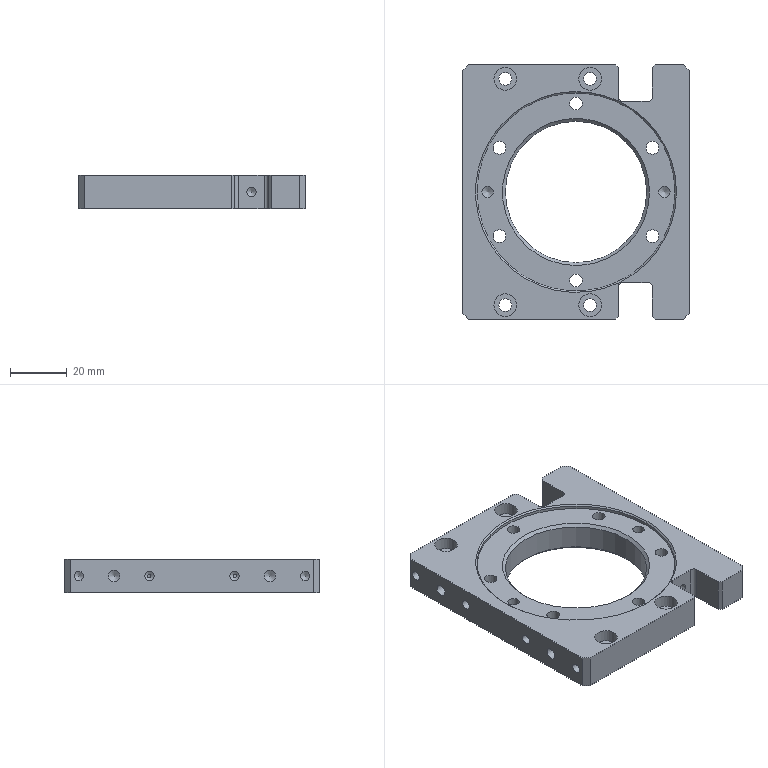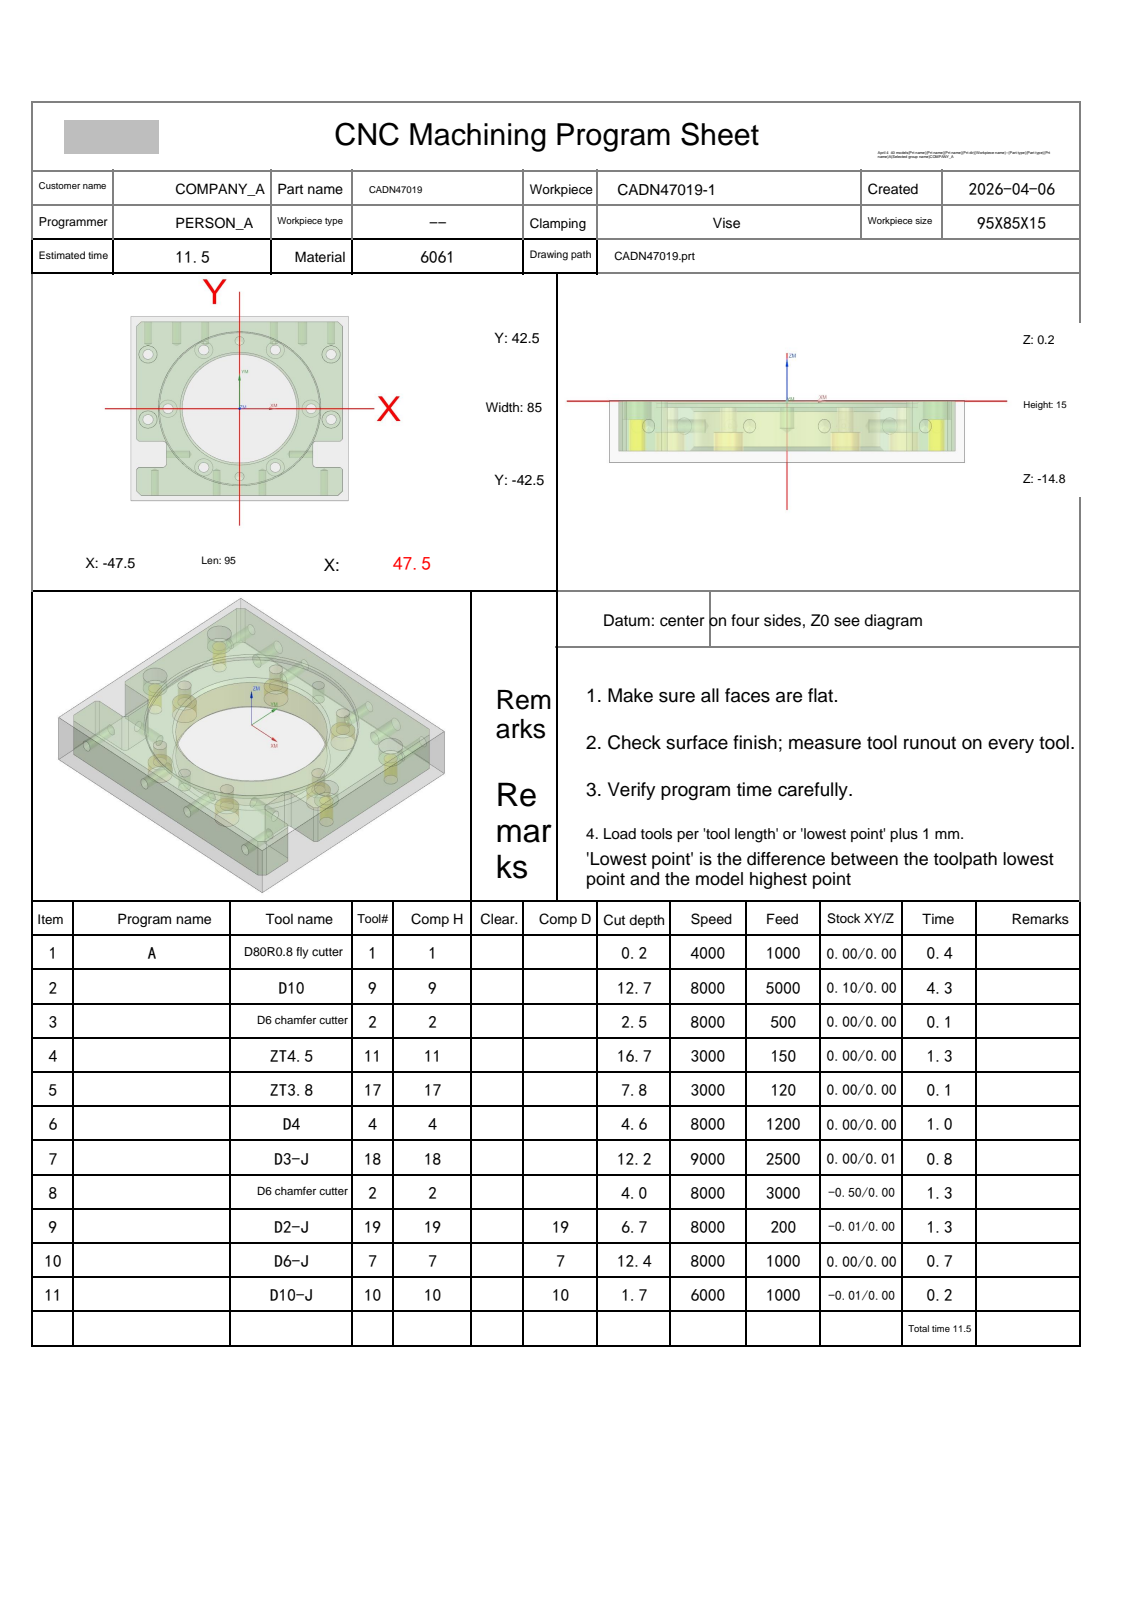NC program | NX | posted by the shop | part box 80 x 90 x 12 mm
Lines 2082 to 3119 of 6628:
N7 T18 M06
(D3-J  D=3. R=0. H=18 ce=0.00 di=0.01)
G00 G90 G54 X37.397 Y-17.082 M03 S9000
G43 H18 Z20.
M08
Z.151
G01 Y-17.076 Z.083 F2000.
X37.394 Y-17.059 Z.021
X37.39 Y-17.032 Z-.034
X37.384 Y-16.996 Z-.083
X37.375 Y-16.954 Z-.125
X37.364 Y-16.907 Z-.163
X37.351 Y-16.856 Z-.195
X37.334 Y-16.803 Z-.222
X37.315 Y-16.749 Z-.244
X37.293 Y-16.696 Z-.262
X37.267 Y-16.646 Z-.276
X37.237 Y-16.6 Z-.287
X37.204 Y-16.559 Z-.294
X37.167 Y-16.525 Z-.297
X37.125 Y-16.5 Z-.299
X33.5 F2500.
Y-20.125
X33.516 Y-20.154 Z-.3
X33.561 Y-20.159 Z-.302
X33.633 Y-20.143 Z-.306
X33.728 Y-20.106 Z-.312
X33.843 Y-20.052 Z-.319
X33.975 Y-19.981 Z-.327
X34.273 Y-19.8 Z-.346
X34.466 Y-19.672 Z-.358
X34.779 Y-19.448 Z-.38
X35.235 Y-19.077 Z-.413
X35.669 Y-18.672 Z-.448
X36.075 Y-18.238 Z-.483
X36.447 Y-17.781 Z-.517
X36.671 Y-17.468 Z-.538
X36.8 Y-17.275 Z-.55
X36.981 Y-16.976 Z-.569
X37.052 Y-16.844 Z-.577
X37.106 Y-16.729 Z-.584
X37.142 Y-16.633 Z-.59
X37.159 Y-16.561 Z-.594
X37.154 Y-16.516 Z-.597
X37.125 Y-16.5 Z-.598
X33.5
Y-20.125
X33.516 Y-20.154
X33.561 Y-20.159 Z-.601
X33.633 Y-20.143 Z-.605
X33.728 Y-20.106 Z-.611
X33.843 Y-20.052 Z-.618
X33.975 Y-19.981 Z-.626
X34.273 Y-19.8 Z-.645
X34.466 Y-19.672 Z-.657
X34.779 Y-19.448 Z-.678
X35.235 Y-19.077 Z-.712
X35.669 Y-18.672 Z-.747
X36.075 Y-18.238 Z-.782
X36.447 Y-17.781 Z-.815
X36.671 Y-17.468 Z-.837
X36.8 Y-17.275 Z-.849
X36.981 Y-16.976 Z-.868
X37.052 Y-16.844 Z-.876
X37.106 Y-16.729 Z-.883
X37.142 Y-16.633 Z-.889
X37.159 Y-16.561 Z-.893
X37.154 Y-16.516 Z-.895
X37.125 Y-16.5 Z-.896
X33.5
Y-20.125
X33.516 Y-20.154 Z-.897
X33.561 Y-20.159 Z-.9
X33.633 Y-20.143 Z-.904
X33.728 Y-20.106 Z-.91
X33.843 Y-20.052 Z-.916
X33.975 Y-19.981 Z-.925
X34.273 Y-19.8 Z-.943
X34.466 Y-19.672 Z-.956
X34.779 Y-19.448 Z-.977
X35.235 Y-19.077 Z-1.011
X35.669 Y-18.672 Z-1.046
X36.075 Y-18.238 Z-1.08
X36.447 Y-17.781 Z-1.114
X36.671 Y-17.468 Z-1.135
X36.8 Y-17.275 Z-1.148
X36.981 Y-16.976 Z-1.167
X37.052 Y-16.844 Z-1.175
X37.106 Y-16.729 Z-1.182
X37.142 Y-16.633 Z-1.187
X37.159 Y-16.561 Z-1.191
X37.154 Y-16.516 Z-1.194
X37.125 Y-16.5 Z-1.195
X33.5
Y-20.125
X33.516 Y-20.154 Z-1.196
X33.561 Y-20.159 Z-1.199
X33.633 Y-20.143 Z-1.203
X33.728 Y-20.106 Z-1.208
X33.843 Y-20.052 Z-1.215
X33.975 Y-19.981 Z-1.223
X34.273 Y-19.8 Z-1.242
X34.466 Y-19.672 Z-1.255
X34.779 Y-19.448 Z-1.276
X35.235 Y-19.077 Z-1.31
X35.669 Y-18.672 Z-1.344
X36.075 Y-18.238 Z-1.379
X36.447 Y-17.781 Z-1.413
X36.671 Y-17.468 Z-1.434
X36.8 Y-17.275 Z-1.447
X36.981 Y-16.976 Z-1.465
X37.052 Y-16.844 Z-1.474
X37.106 Y-16.729 Z-1.48
X37.142 Y-16.633 Z-1.486
X37.159 Y-16.561 Z-1.49
X37.154 Y-16.516 Z-1.493
X37.125 Y-16.5 Z-1.494
X33.5
Y-20.125
X33.516 Y-20.154 Z-1.495
X33.561 Y-20.159 Z-1.497
X33.633 Y-20.143 Z-1.501
X33.728 Y-20.106 Z-1.507
X33.843 Y-20.052 Z-1.514
X33.975 Y-19.981 Z-1.522
X34.273 Y-19.8 Z-1.541
X34.466 Y-19.672 Z-1.553
X34.779 Y-19.448 Z-1.575
X35.235 Y-19.077 Z-1.608
X35.669 Y-18.672 Z-1.643
X36.075 Y-18.238 Z-1.678
X36.447 Y-17.781 Z-1.712
X36.671 Y-17.468 Z-1.733
X36.8 Y-17.275 Z-1.745
X36.981 Y-16.976 Z-1.764
X37.052 Y-16.844 Z-1.772
X37.106 Y-16.729 Z-1.779
X37.142 Y-16.633 Z-1.785
X37.159 Y-16.561 Z-1.789
X37.154 Y-16.516 Z-1.792
X37.125 Y-16.5 Z-1.793
X33.5
Y-20.125
X33.516 Y-20.154
X33.561 Y-20.159 Z-1.796
X33.633 Y-20.143 Z-1.8
X33.728 Y-20.106 Z-1.806
X33.843 Y-20.052 Z-1.813
X33.975 Y-19.981 Z-1.821
X34.273 Y-19.8 Z-1.84
X34.466 Y-19.672 Z-1.852
X34.779 Y-19.448 Z-1.873
X35.235 Y-19.077 Z-1.907
X35.669 Y-18.672 Z-1.942
X36.075 Y-18.238 Z-1.977
X36.447 Y-17.781 Z-2.01
X36.671 Y-17.468 Z-2.032
X36.8 Y-17.275 Z-2.044
X36.981 Y-16.976 Z-2.063
X37.052 Y-16.844 Z-2.071
X37.106 Y-16.729 Z-2.078
X37.142 Y-16.633 Z-2.084
X37.159 Y-16.561 Z-2.088
X37.154 Y-16.516 Z-2.09
X37.125 Y-16.5 Z-2.091
X33.5
Y-20.125
X33.516 Y-20.154 Z-2.092
X33.561 Y-20.159 Z-2.095
X33.633 Y-20.143 Z-2.099
X33.728 Y-20.106 Z-2.105
X33.843 Y-20.052 Z-2.111
X33.975 Y-19.981 Z-2.12
X34.273 Y-19.8 Z-2.138
X34.466 Y-19.672 Z-2.151
X34.779 Y-19.448 Z-2.172
X35.235 Y-19.077 Z-2.206
X35.669 Y-18.672 Z-2.241
X36.075 Y-18.238 Z-2.275
X36.447 Y-17.781 Z-2.309
X36.671 Y-17.468 Z-2.33
X36.8 Y-17.275 Z-2.343
X36.981 Y-16.976 Z-2.362
X37.052 Y-16.844 Z-2.37
X37.106 Y-16.729 Z-2.377
X37.142 Y-16.633 Z-2.382
X37.159 Y-16.561 Z-2.386
X37.154 Y-16.516 Z-2.389
X37.125 Y-16.5 Z-2.39
X33.5
Y-20.125
X33.516 Y-20.154 Z-2.391
X33.561 Y-20.159 Z-2.394
X33.633 Y-20.143 Z-2.398
X33.728 Y-20.106 Z-2.403
X33.843 Y-20.052 Z-2.41
X33.975 Y-19.981 Z-2.418
X34.273 Y-19.8 Z-2.437
X34.466 Y-19.672 Z-2.45
X34.779 Y-19.448 Z-2.471
X35.235 Y-19.077 Z-2.505
X35.669 Y-18.672 Z-2.539
X36.075 Y-18.238 Z-2.574
X36.447 Y-17.781 Z-2.608
X36.671 Y-17.468 Z-2.629
X36.8 Y-17.275 Z-2.642
X36.981 Y-16.976 Z-2.66
X37.052 Y-16.844 Z-2.669
X37.106 Y-16.729 Z-2.675
X37.142 Y-16.633 Z-2.681
X37.159 Y-16.561 Z-2.685
X37.154 Y-16.516 Z-2.688
X37.125 Y-16.5 Z-2.689
X33.5
Y-20.125
X33.516 Y-20.154 Z-2.69
X33.561 Y-20.159 Z-2.692
X33.633 Y-20.143 Z-2.696
X33.728 Y-20.106 Z-2.702
X33.843 Y-20.052 Z-2.709
X33.975 Y-19.981 Z-2.717
X34.273 Y-19.8 Z-2.736
X34.466 Y-19.672 Z-2.748
X34.779 Y-19.448 Z-2.77
X35.235 Y-19.077 Z-2.803
X35.669 Y-18.672 Z-2.838
X36.075 Y-18.238 Z-2.873
X36.447 Y-17.781 Z-2.907
X36.671 Y-17.468 Z-2.928
X36.8 Y-17.275 Z-2.94
X36.981 Y-16.976 Z-2.959
X37.052 Y-16.844 Z-2.967
X37.106 Y-16.729 Z-2.974
X37.142 Y-16.633 Z-2.98
X37.159 Y-16.561 Z-2.984
X37.154 Y-16.516 Z-2.987
X37.125 Y-16.5 Z-2.988
X33.5
Y-20.125
X33.516 Y-20.154
X33.561 Y-20.159 Z-2.991
X33.633 Y-20.143 Z-2.995
X33.728 Y-20.106 Z-3.001
X33.843 Y-20.052 Z-3.008
X33.975 Y-19.981 Z-3.016
X34.273 Y-19.8 Z-3.035
X34.466 Y-19.672 Z-3.047
X34.779 Y-19.448 Z-3.068
X35.235 Y-19.077 Z-3.102
X35.669 Y-18.672 Z-3.137
X36.075 Y-18.238 Z-3.172
X36.447 Y-17.781 Z-3.205
X36.671 Y-17.468 Z-3.227
X36.8 Y-17.275 Z-3.239
X36.981 Y-16.976 Z-3.258
X37.052 Y-16.844 Z-3.266
X37.106 Y-16.729 Z-3.273
X37.142 Y-16.633 Z-3.279
X37.159 Y-16.561 Z-3.283
X37.154 Y-16.516 Z-3.285
X37.125 Y-16.5 Z-3.286
X33.5
Y-20.125
X33.516 Y-20.154 Z-3.287
X33.561 Y-20.159 Z-3.29
X33.633 Y-20.143 Z-3.294
X33.728 Y-20.106 Z-3.3
X33.843 Y-20.052 Z-3.306
X33.975 Y-19.981 Z-3.315
X34.273 Y-19.8 Z-3.333
X34.466 Y-19.672 Z-3.346
X34.779 Y-19.448 Z-3.367
X35.235 Y-19.077 Z-3.401
X35.669 Y-18.672 Z-3.436
X36.075 Y-18.238 Z-3.47
X36.447 Y-17.781 Z-3.504
X36.671 Y-17.468 Z-3.525
X36.8 Y-17.275 Z-3.538
X36.981 Y-16.976 Z-3.557
X37.052 Y-16.844 Z-3.565
X37.106 Y-16.729 Z-3.572
X37.142 Y-16.633 Z-3.577
X37.159 Y-16.561 Z-3.581
X37.154 Y-16.516 Z-3.584
X37.125 Y-16.5 Z-3.585
X33.5
Y-20.125
X33.516 Y-20.154 Z-3.586
X33.561 Y-20.159 Z-3.589
X33.633 Y-20.143 Z-3.593
X33.728 Y-20.106 Z-3.598
X33.843 Y-20.052 Z-3.605
X33.975 Y-19.981 Z-3.613
X34.273 Y-19.8 Z-3.632
X34.466 Y-19.672 Z-3.645
X34.779 Y-19.448 Z-3.666
X35.235 Y-19.077 Z-3.7
X35.669 Y-18.672 Z-3.734
X36.075 Y-18.238 Z-3.769
X36.447 Y-17.781 Z-3.803
X36.671 Y-17.468 Z-3.824
X36.8 Y-17.275 Z-3.837
X36.981 Y-16.976 Z-3.855
X37.052 Y-16.844 Z-3.864
X37.106 Y-16.729 Z-3.87
X37.142 Y-16.633 Z-3.876
X37.159 Y-16.561 Z-3.88
X37.154 Y-16.516 Z-3.883
X37.125 Y-16.5 Z-3.884
X33.5
Y-20.125
X33.516 Y-20.154 Z-3.885
X33.561 Y-20.159 Z-3.887
X33.633 Y-20.143 Z-3.891
X33.728 Y-20.106 Z-3.897
X33.843 Y-20.052 Z-3.904
X33.975 Y-19.981 Z-3.912
X34.273 Y-19.8 Z-3.931
X34.466 Y-19.672 Z-3.943
X34.779 Y-19.448 Z-3.965
X35.235 Y-19.077 Z-3.998
X35.669 Y-18.672 Z-4.033
X36.075 Y-18.238 Z-4.068
X36.447 Y-17.781 Z-4.102
X36.671 Y-17.468 Z-4.123
X36.8 Y-17.275 Z-4.135
X36.981 Y-16.976 Z-4.154
X37.052 Y-16.844 Z-4.162
X37.106 Y-16.729 Z-4.169
X37.142 Y-16.633 Z-4.175
X37.159 Y-16.561 Z-4.179
X37.154 Y-16.516 Z-4.182
X37.125 Y-16.5 Z-4.183
X33.5
Y-20.125
X33.516 Y-20.154
X33.561 Y-20.159 Z-4.186
X33.633 Y-20.143 Z-4.19
X33.728 Y-20.106 Z-4.196
X33.843 Y-20.052 Z-4.203
X33.975 Y-19.981 Z-4.211
X34.273 Y-19.8 Z-4.23
X34.466 Y-19.672 Z-4.242
X34.779 Y-19.448 Z-4.263
X35.235 Y-19.077 Z-4.297
X35.669 Y-18.672 Z-4.332
X36.075 Y-18.238 Z-4.367
X36.447 Y-17.781 Z-4.4
X36.671 Y-17.468 Z-4.422
X36.8 Y-17.275 Z-4.434
X36.981 Y-16.976 Z-4.453
X37.052 Y-16.844 Z-4.461
X37.106 Y-16.729 Z-4.468
X37.142 Y-16.633 Z-4.474
X37.159 Y-16.561 Z-4.478
X37.154 Y-16.516 Z-4.48
X37.125 Y-16.5 Z-4.481
X33.5
Y-20.125
X33.516 Y-20.154 Z-4.482
X33.561 Y-20.159 Z-4.485
X33.633 Y-20.143 Z-4.489
X33.728 Y-20.106 Z-4.495
X33.843 Y-20.052 Z-4.501
X33.975 Y-19.981 Z-4.51
X34.273 Y-19.8 Z-4.528
X34.466 Y-19.672 Z-4.541
X34.779 Y-19.448 Z-4.562
X35.235 Y-19.077 Z-4.596
X35.669 Y-18.672 Z-4.631
X36.075 Y-18.238 Z-4.665
X36.447 Y-17.781 Z-4.699
X36.671 Y-17.468 Z-4.72
X36.8 Y-17.275 Z-4.733
X36.981 Y-16.976 Z-4.752
X37.052 Y-16.844 Z-4.76
X37.106 Y-16.729 Z-4.767
X37.142 Y-16.633 Z-4.772
X37.159 Y-16.561 Z-4.776
X37.154 Y-16.516 Z-4.779
X37.125 Y-16.5 Z-4.78
X33.5
Y-20.125
X33.516 Y-20.154 Z-4.781
X33.561 Y-20.159 Z-4.784
X33.633 Y-20.143 Z-4.788
X33.728 Y-20.106 Z-4.793
X33.843 Y-20.052 Z-4.8
X33.975 Y-19.981 Z-4.808
X34.273 Y-19.8 Z-4.827
X34.466 Y-19.672 Z-4.84
X34.779 Y-19.448 Z-4.861
X35.235 Y-19.077 Z-4.895
X35.669 Y-18.672 Z-4.929
X36.075 Y-18.238 Z-4.964
X36.447 Y-17.781 Z-4.998
X36.671 Y-17.468 Z-5.019
X36.8 Y-17.275 Z-5.032
X36.981 Y-16.976 Z-5.05
X37.052 Y-16.844 Z-5.059
X37.106 Y-16.729 Z-5.065
X37.142 Y-16.633 Z-5.071
X37.159 Y-16.561 Z-5.075
X37.154 Y-16.516 Z-5.078
X37.125 Y-16.5 Z-5.079
X33.5
Y-20.125
X33.516 Y-20.154 Z-5.08
X33.561 Y-20.159 Z-5.082
X33.633 Y-20.143 Z-5.086
X33.728 Y-20.106 Z-5.092
X33.843 Y-20.052 Z-5.099
X33.975 Y-19.981 Z-5.107
X34.273 Y-19.8 Z-5.126
X34.466 Y-19.672 Z-5.138
X34.779 Y-19.448 Z-5.16
X35.235 Y-19.077 Z-5.193
X35.669 Y-18.672 Z-5.228
X36.075 Y-18.238 Z-5.263
X36.447 Y-17.781 Z-5.297
X36.671 Y-17.468 Z-5.318
X36.8 Y-17.275 Z-5.33
X36.981 Y-16.976 Z-5.349
X37.052 Y-16.844 Z-5.357
X37.106 Y-16.729 Z-5.364
X37.142 Y-16.633 Z-5.37
X37.159 Y-16.561 Z-5.374
X37.154 Y-16.516 Z-5.377
X37.125 Y-16.5 Z-5.378
X33.5
Y-20.125
X33.516 Y-20.154
X33.561 Y-20.159 Z-5.381
X33.633 Y-20.143 Z-5.385
X33.728 Y-20.106 Z-5.391
X33.843 Y-20.052 Z-5.398
X33.975 Y-19.981 Z-5.406
X34.273 Y-19.8 Z-5.425
X34.466 Y-19.672 Z-5.437
X34.779 Y-19.448 Z-5.458
X35.235 Y-19.077 Z-5.492
X35.669 Y-18.672 Z-5.527
X36.075 Y-18.238 Z-5.562
X36.447 Y-17.781 Z-5.595
X36.671 Y-17.468 Z-5.617
X36.8 Y-17.275 Z-5.629
X36.981 Y-16.976 Z-5.648
X37.052 Y-16.844 Z-5.656
X37.106 Y-16.729 Z-5.663
X37.142 Y-16.633 Z-5.669
X37.159 Y-16.561 Z-5.673
X37.154 Y-16.516 Z-5.675
X37.125 Y-16.5 Z-5.676
X33.5
Y-20.125
X33.516 Y-20.154 Z-5.677
X33.561 Y-20.159 Z-5.68
X33.633 Y-20.143 Z-5.684
X33.728 Y-20.106 Z-5.69
X33.843 Y-20.052 Z-5.696
X33.975 Y-19.981 Z-5.705
X34.273 Y-19.8 Z-5.723
X34.466 Y-19.672 Z-5.736
X34.779 Y-19.448 Z-5.757
X35.235 Y-19.077 Z-5.791
X35.669 Y-18.672 Z-5.826
X36.075 Y-18.238 Z-5.86
X36.447 Y-17.781 Z-5.894
X36.671 Y-17.468 Z-5.915
X36.8 Y-17.275 Z-5.928
X36.981 Y-16.976 Z-5.947
X37.052 Y-16.844 Z-5.955
X37.106 Y-16.729 Z-5.962
X37.142 Y-16.633 Z-5.967
X37.159 Y-16.561 Z-5.971
X37.154 Y-16.516 Z-5.974
X37.125 Y-16.5 Z-5.975
X33.5
Y-20.125
X33.516 Y-20.154 Z-5.976
X33.561 Y-20.159 Z-5.979
X33.633 Y-20.143 Z-5.983
X33.728 Y-20.106 Z-5.988
X33.843 Y-20.052 Z-5.995
X33.975 Y-19.981 Z-6.003
X34.273 Y-19.8 Z-6.022
X34.466 Y-19.672 Z-6.035
X34.779 Y-19.448 Z-6.056
X35.235 Y-19.077 Z-6.09
X35.669 Y-18.672 Z-6.124
X36.075 Y-18.238 Z-6.159
X36.447 Y-17.781 Z-6.193
X36.671 Y-17.468 Z-6.214
X36.8 Y-17.275 Z-6.227
X36.981 Y-16.976 Z-6.245
X37.052 Y-16.844 Z-6.254
X37.106 Y-16.729 Z-6.26
X37.142 Y-16.633 Z-6.266
X37.159 Y-16.561 Z-6.27
X37.154 Y-16.516 Z-6.273
X37.125 Y-16.5 Z-6.274
X33.5
Y-20.125
X33.516 Y-20.154 Z-6.275
X33.561 Y-20.159 Z-6.277
X33.633 Y-20.143 Z-6.281
X33.728 Y-20.106 Z-6.287
X33.843 Y-20.052 Z-6.294
X33.975 Y-19.981 Z-6.302
X34.273 Y-19.8 Z-6.321
X34.466 Y-19.672 Z-6.333
X34.779 Y-19.448 Z-6.355
X35.235 Y-19.077 Z-6.388
X35.669 Y-18.672 Z-6.423
X36.075 Y-18.238 Z-6.458
X36.447 Y-17.781 Z-6.492
X36.671 Y-17.468 Z-6.513
X36.8 Y-17.275 Z-6.525
X36.981 Y-16.976 Z-6.544
X37.052 Y-16.844 Z-6.552
X37.106 Y-16.729 Z-6.559
X37.142 Y-16.633 Z-6.565
X37.159 Y-16.561 Z-6.569
X37.154 Y-16.516 Z-6.572
X37.125 Y-16.5 Z-6.573
X33.5
Y-20.125
X33.516 Y-20.154
X33.561 Y-20.159 Z-6.576
X33.633 Y-20.143 Z-6.58
X33.728 Y-20.106 Z-6.586
X33.843 Y-20.052 Z-6.593
X33.975 Y-19.981 Z-6.601
X34.273 Y-19.8 Z-6.62
X34.466 Y-19.672 Z-6.632
X34.779 Y-19.448 Z-6.653
X35.235 Y-19.077 Z-6.687
X35.669 Y-18.672 Z-6.722
X36.075 Y-18.238 Z-6.757
X36.447 Y-17.781 Z-6.79
X36.671 Y-17.468 Z-6.812
X36.8 Y-17.275 Z-6.824
X36.981 Y-16.976 Z-6.843
X37.052 Y-16.844 Z-6.851
X37.106 Y-16.729 Z-6.858
X37.142 Y-16.633 Z-6.864
X37.159 Y-16.561 Z-6.868
X37.154 Y-16.516 Z-6.87
X37.125 Y-16.5 Z-6.871
X33.5
Y-20.125
X33.516 Y-20.154 Z-6.872
X33.561 Y-20.159 Z-6.875
X33.633 Y-20.143 Z-6.879
X33.728 Y-20.106 Z-6.885
X33.843 Y-20.052 Z-6.891
X33.975 Y-19.981 Z-6.9
X34.273 Y-19.8 Z-6.918
X34.466 Y-19.672 Z-6.931
X34.779 Y-19.448 Z-6.952
X35.235 Y-19.077 Z-6.986
X35.669 Y-18.672 Z-7.021
X36.075 Y-18.238 Z-7.055
X36.447 Y-17.781 Z-7.089
X36.671 Y-17.468 Z-7.11
X36.8 Y-17.275 Z-7.123
X36.981 Y-16.976 Z-7.142
X37.052 Y-16.844 Z-7.15
X37.106 Y-16.729 Z-7.157
X37.142 Y-16.633 Z-7.162
X37.159 Y-16.561 Z-7.166
X37.154 Y-16.516 Z-7.169
X37.125 Y-16.5 Z-7.17
X33.5
Y-20.125
X33.516 Y-20.154 Z-7.171
X33.561 Y-20.159 Z-7.174
X33.633 Y-20.143 Z-7.178
X33.728 Y-20.106 Z-7.183
X33.843 Y-20.052 Z-7.19
X33.975 Y-19.981 Z-7.198
X34.273 Y-19.8 Z-7.217
X34.466 Y-19.672 Z-7.23
X34.779 Y-19.448 Z-7.251
X35.235 Y-19.077 Z-7.285
X35.669 Y-18.672 Z-7.319
X36.075 Y-18.238 Z-7.354
X36.447 Y-17.781 Z-7.388
X36.671 Y-17.468 Z-7.409
X36.8 Y-17.275 Z-7.422
X36.981 Y-16.976 Z-7.44
X37.052 Y-16.844 Z-7.449
X37.106 Y-16.729 Z-7.455
X37.142 Y-16.633 Z-7.461
X37.159 Y-16.561 Z-7.465
X37.154 Y-16.516 Z-7.468
X37.125 Y-16.5 Z-7.469
X33.5
Y-20.125
X33.516 Y-20.154 Z-7.47
X33.561 Y-20.159 Z-7.472
X33.633 Y-20.143 Z-7.476
X33.728 Y-20.106 Z-7.482
X33.843 Y-20.052 Z-7.489
X33.975 Y-19.981 Z-7.497
X34.273 Y-19.8 Z-7.516
X34.466 Y-19.672 Z-7.528
X34.779 Y-19.448 Z-7.55
X35.235 Y-19.077 Z-7.583
X35.669 Y-18.672 Z-7.618
X36.075 Y-18.238 Z-7.653
X36.447 Y-17.781 Z-7.687
X36.671 Y-17.468 Z-7.708
X36.8 Y-17.275 Z-7.72
X36.981 Y-16.976 Z-7.739
X37.052 Y-16.844 Z-7.747
X37.106 Y-16.729 Z-7.754
X37.142 Y-16.633 Z-7.76
X37.159 Y-16.561 Z-7.764
X37.154 Y-16.516 Z-7.767
X37.125 Y-16.5 Z-7.768
X33.5
Y-20.125
X33.516 Y-20.154
X33.561 Y-20.159 Z-7.771
X33.633 Y-20.143 Z-7.775
X33.728 Y-20.106 Z-7.781
X33.843 Y-20.052 Z-7.788
X33.975 Y-19.981 Z-7.796
X34.273 Y-19.8 Z-7.815
X34.466 Y-19.672 Z-7.827
X34.779 Y-19.448 Z-7.848
X35.235 Y-19.077 Z-7.882
X35.669 Y-18.672 Z-7.917
X36.075 Y-18.238 Z-7.952
X36.447 Y-17.781 Z-7.985
X36.671 Y-17.468 Z-8.007
X36.8 Y-17.275 Z-8.019
X36.981 Y-16.976 Z-8.038
X37.052 Y-16.844 Z-8.046
X37.106 Y-16.729 Z-8.053
X37.142 Y-16.633 Z-8.059
X37.159 Y-16.561 Z-8.063
X37.154 Y-16.516 Z-8.065
X37.125 Y-16.5 Z-8.066
X33.5
Y-20.125
X33.516 Y-20.154 Z-8.067
X33.561 Y-20.159 Z-8.07
X33.633 Y-20.143 Z-8.074
X33.728 Y-20.106 Z-8.08
X33.843 Y-20.052 Z-8.086
X33.975 Y-19.981 Z-8.095
X34.273 Y-19.8 Z-8.113
X34.466 Y-19.672 Z-8.126
X34.779 Y-19.448 Z-8.147
X35.235 Y-19.077 Z-8.181
X35.669 Y-18.672 Z-8.216
X36.075 Y-18.238 Z-8.25
X36.447 Y-17.781 Z-8.284
X36.671 Y-17.468 Z-8.305
X36.8 Y-17.275 Z-8.318
X36.981 Y-16.976 Z-8.337
X37.052 Y-16.844 Z-8.345
X37.106 Y-16.729 Z-8.352
X37.142 Y-16.633 Z-8.357
X37.159 Y-16.561 Z-8.361
X37.154 Y-16.516 Z-8.364
X37.125 Y-16.5 Z-8.365
X33.5
Y-20.125
X33.516 Y-20.154 Z-8.366
X33.561 Y-20.159 Z-8.369
X33.633 Y-20.143 Z-8.373
X33.728 Y-20.106 Z-8.378
X33.843 Y-20.052 Z-8.385
X33.975 Y-19.981 Z-8.393
X34.273 Y-19.8 Z-8.412
X34.466 Y-19.672 Z-8.425
X34.779 Y-19.448 Z-8.446
X35.235 Y-19.077 Z-8.48
X35.669 Y-18.672 Z-8.514
X36.075 Y-18.238 Z-8.549
X36.447 Y-17.781 Z-8.583
X36.671 Y-17.468 Z-8.604
X36.8 Y-17.275 Z-8.617
X36.981 Y-16.976 Z-8.635
X37.052 Y-16.844 Z-8.644
X37.106 Y-16.729 Z-8.65
X37.142 Y-16.633 Z-8.656
X37.159 Y-16.561 Z-8.66
X37.154 Y-16.516 Z-8.663
X37.125 Y-16.5 Z-8.664
X33.5
Y-20.125
X33.516 Y-20.154 Z-8.665
X33.561 Y-20.159 Z-8.667
X33.633 Y-20.143 Z-8.671
X33.728 Y-20.106 Z-8.677
X33.843 Y-20.052 Z-8.684
X33.975 Y-19.981 Z-8.692
X34.273 Y-19.8 Z-8.711
X34.466 Y-19.672 Z-8.723
X34.779 Y-19.448 Z-8.745
X35.235 Y-19.077 Z-8.778
X35.669 Y-18.672 Z-8.813
X36.075 Y-18.238 Z-8.848
X36.447 Y-17.781 Z-8.882
X36.671 Y-17.468 Z-8.903
X36.8 Y-17.275 Z-8.915
X36.981 Y-16.976 Z-8.934
X37.052 Y-16.844 Z-8.942
X37.106 Y-16.729 Z-8.949
X37.142 Y-16.633 Z-8.955
X37.159 Y-16.561 Z-8.959
X37.154 Y-16.516 Z-8.962
X37.125 Y-16.5 Z-8.963
X33.5
Y-20.125
X33.516 Y-20.154
X33.561 Y-20.159 Z-8.966
X33.633 Y-20.143 Z-8.97
X33.728 Y-20.106 Z-8.976
X33.843 Y-20.052 Z-8.983
X33.975 Y-19.981 Z-8.991
X34.273 Y-19.8 Z-9.01
X34.466 Y-19.672 Z-9.022
X34.779 Y-19.448 Z-9.043
X35.235 Y-19.077 Z-9.077
X35.669 Y-18.672 Z-9.112
X36.075 Y-18.238 Z-9.147
X36.447 Y-17.781 Z-9.18
X36.671 Y-17.468 Z-9.202
X36.8 Y-17.275 Z-9.214
X36.981 Y-16.976 Z-9.233
X37.052 Y-16.844 Z-9.241
X37.106 Y-16.729 Z-9.248
X37.142 Y-16.633 Z-9.254
X37.159 Y-16.561 Z-9.258
X37.154 Y-16.516 Z-9.26
X37.125 Y-16.5 Z-9.261
X33.5
Y-20.125
X33.516 Y-20.154 Z-9.262
X33.561 Y-20.159 Z-9.265
X33.633 Y-20.143 Z-9.269
X33.728 Y-20.106 Z-9.275
X33.843 Y-20.052 Z-9.281
X33.975 Y-19.981 Z-9.29
X34.273 Y-19.8 Z-9.308
X34.466 Y-19.672 Z-9.321
X34.779 Y-19.448 Z-9.342
X35.235 Y-19.077 Z-9.376
X35.669 Y-18.672 Z-9.411
X36.075 Y-18.238 Z-9.445
X36.447 Y-17.781 Z-9.479
X36.671 Y-17.468 Z-9.5
X36.8 Y-17.275 Z-9.513
X36.981 Y-16.976 Z-9.532
X37.052 Y-16.844 Z-9.54
X37.106 Y-16.729 Z-9.547
X37.142 Y-16.633 Z-9.552
X37.159 Y-16.561 Z-9.556
X37.154 Y-16.516 Z-9.559
X37.125 Y-16.5 Z-9.56
X33.5
Y-20.125
X33.516 Y-20.154 Z-9.561
X33.561 Y-20.159 Z-9.564
X33.633 Y-20.143 Z-9.568
X33.728 Y-20.106 Z-9.573
X33.843 Y-20.052 Z-9.58
X33.975 Y-19.981 Z-9.588
X34.273 Y-19.8 Z-9.607
X34.466 Y-19.672 Z-9.62
X34.779 Y-19.448 Z-9.641
X35.235 Y-19.077 Z-9.675
X35.669 Y-18.672 Z-9.709
X36.075 Y-18.238 Z-9.744
X36.447 Y-17.781 Z-9.778
X36.671 Y-17.468 Z-9.799
X36.8 Y-17.275 Z-9.812
X36.981 Y-16.976 Z-9.83
X37.052 Y-16.844 Z-9.839
X37.106 Y-16.729 Z-9.845
X37.142 Y-16.633 Z-9.851
X37.159 Y-16.561 Z-9.855
X37.154 Y-16.516 Z-9.858
X37.125 Y-16.5 Z-9.859
X33.5
Y-20.125
X33.516 Y-20.154 Z-9.86
X33.561 Y-20.159 Z-9.862
X33.633 Y-20.143 Z-9.866
X33.728 Y-20.106 Z-9.872
X33.843 Y-20.052 Z-9.879
X33.975 Y-19.981 Z-9.887
X34.273 Y-19.8 Z-9.906
X34.466 Y-19.672 Z-9.918
X34.779 Y-19.448 Z-9.94
X35.235 Y-19.077 Z-9.973
X35.669 Y-18.672 Z-10.008
X36.075 Y-18.238 Z-10.043
X36.447 Y-17.781 Z-10.077
X36.671 Y-17.468 Z-10.098
X36.8 Y-17.275 Z-10.11
X36.981 Y-16.976 Z-10.129
X37.052 Y-16.844 Z-10.137
X37.106 Y-16.729 Z-10.144
X37.142 Y-16.633 Z-10.15
X37.159 Y-16.561 Z-10.154
X37.154 Y-16.516 Z-10.157
X37.125 Y-16.5 Z-10.158
X33.5
Y-20.125
X33.516 Y-20.154
X33.561 Y-20.159 Z-10.161
X33.633 Y-20.143 Z-10.165
X33.728 Y-20.106 Z-10.171
X33.843 Y-20.052 Z-10.178
X33.975 Y-19.981 Z-10.186
X34.273 Y-19.8 Z-10.205
X34.466 Y-19.672 Z-10.217
X34.779 Y-19.448 Z-10.238
X35.235 Y-19.077 Z-10.272
X35.669 Y-18.672 Z-10.307
X36.075 Y-18.238 Z-10.342
X36.447 Y-17.781 Z-10.375
X36.671 Y-17.468 Z-10.397
X36.8 Y-17.275 Z-10.409
X36.981 Y-16.976 Z-10.428
X37.052 Y-16.844 Z-10.436
X37.106 Y-16.729 Z-10.443
X37.142 Y-16.633 Z-10.449
X37.159 Y-16.561 Z-10.453
X37.154 Y-16.516 Z-10.455
X37.125 Y-16.5 Z-10.456
X33.5
Y-20.125
X33.516 Y-20.154 Z-10.457
X33.561 Y-20.159 Z-10.46
X33.633 Y-20.143 Z-10.464
X33.728 Y-20.106 Z-10.47
X33.843 Y-20.052 Z-10.476
X33.975 Y-19.981 Z-10.485
X34.273 Y-19.8 Z-10.503
X34.466 Y-19.672 Z-10.516
X34.779 Y-19.448 Z-10.537
X35.235 Y-19.077 Z-10.571
X35.669 Y-18.672 Z-10.606
X36.075 Y-18.238 Z-10.64
X36.447 Y-17.781 Z-10.674
X36.671 Y-17.468 Z-10.695
X36.8 Y-17.275 Z-10.708
X36.981 Y-16.976 Z-10.727
X37.052 Y-16.844 Z-10.735
X37.106 Y-16.729 Z-10.742
X37.142 Y-16.633 Z-10.747
X37.159 Y-16.561 Z-10.751
X37.154 Y-16.516 Z-10.754
X37.125 Y-16.5 Z-10.755
X33.5
Y-20.125
X33.516 Y-20.154 Z-10.756
X33.561 Y-20.159 Z-10.759
X33.633 Y-20.143 Z-10.763
X33.728 Y-20.106 Z-10.768
X33.843 Y-20.052 Z-10.775
X33.975 Y-19.981 Z-10.783
X34.273 Y-19.8 Z-10.802
X34.466 Y-19.672 Z-10.815
X34.779 Y-19.448 Z-10.836
X35.235 Y-19.077 Z-10.87
X35.669 Y-18.672 Z-10.904
X36.075 Y-18.238 Z-10.939
X36.447 Y-17.781 Z-10.973
X36.671 Y-17.468 Z-10.994
X36.8 Y-17.275 Z-11.007
X36.981 Y-16.976 Z-11.025
X37.052 Y-16.844 Z-11.034
X37.106 Y-16.729 Z-11.04
X37.142 Y-16.633 Z-11.046
X37.159 Y-16.561 Z-11.05
X37.154 Y-16.516 Z-11.053
X37.125 Y-16.5 Z-11.054
X33.5
Y-20.125
X33.516 Y-20.154 Z-11.055
X33.561 Y-20.159 Z-11.057
X33.633 Y-20.143 Z-11.061
X33.728 Y-20.106 Z-11.067
X33.843 Y-20.052 Z-11.074
X33.975 Y-19.981 Z-11.082
X34.273 Y-19.8 Z-11.101
X34.466 Y-19.672 Z-11.113
X34.779 Y-19.448 Z-11.135
X35.235 Y-19.077 Z-11.168
X35.669 Y-18.672 Z-11.203
X36.075 Y-18.238 Z-11.238
X36.447 Y-17.781 Z-11.272
X36.671 Y-17.468 Z-11.293
X36.8 Y-17.275 Z-11.305
X36.981 Y-16.976 Z-11.324
X37.052 Y-16.844 Z-11.332
X37.106 Y-16.729 Z-11.339
X37.142 Y-16.633 Z-11.345
X37.159 Y-16.561 Z-11.349
X37.154 Y-16.516 Z-11.352
X37.125 Y-16.5 Z-11.353
X33.5
Y-20.125
X33.516 Y-20.154
X33.561 Y-20.159 Z-11.356
X33.633 Y-20.143 Z-11.36
X33.728 Y-20.106 Z-11.366
X33.843 Y-20.052 Z-11.373
X33.975 Y-19.981 Z-11.381
X34.273 Y-19.8 Z-11.4
X34.466 Y-19.672 Z-11.412
X34.779 Y-19.448 Z-11.433
X35.235 Y-19.077 Z-11.467
X35.669 Y-18.672 Z-11.502
X36.075 Y-18.238 Z-11.537
X36.447 Y-17.781 Z-11.57
X36.671 Y-17.468 Z-11.592
X36.8 Y-17.275 Z-11.604
X36.981 Y-16.976 Z-11.623
X37.052 Y-16.844 Z-11.631
X37.106 Y-16.729 Z-11.638
X37.142 Y-16.633 Z-11.644
X37.159 Y-16.561 Z-11.648
X37.154 Y-16.516 Z-11.65
X37.125 Y-16.5 Z-11.651
X33.5
Y-20.125
X33.516 Y-20.154 Z-11.652
X33.561 Y-20.159 Z-11.655
X33.633 Y-20.143 Z-11.659
X33.728 Y-20.106 Z-11.665
X33.843 Y-20.052 Z-11.671
X33.975 Y-19.981 Z-11.68
X34.273 Y-19.8 Z-11.698
X34.466 Y-19.672 Z-11.711
X34.779 Y-19.448 Z-11.732
X35.235 Y-19.077 Z-11.766
X35.669 Y-18.672 Z-11.801
X36.075 Y-18.238 Z-11.835
X36.447 Y-17.781 Z-11.869
X36.671 Y-17.468 Z-11.89
X36.8 Y-17.275 Z-11.903
X36.981 Y-16.976 Z-11.922
X37.052 Y-16.844 Z-11.93
X37.106 Y-16.729 Z-11.937
X37.142 Y-16.633 Z-11.942
X37.159 Y-16.561 Z-11.946
X37.154 Y-16.516 Z-11.949
X37.125 Y-16.5 Z-11.95
X33.5
Y-20.125
X33.525 Y-20.167 Z-11.949
X33.559 Y-20.204 Z-11.945
X33.599 Y-20.237 Z-11.938
X33.645 Y-20.267 Z-11.927
X33.695 Y-20.292 Z-11.913
X33.747 Y-20.315 Z-11.895
X33.8 Y-20.334 Z-11.873
X33.853 Y-20.351 Z-11.846
X33.903 Y-20.364 Z-11.814
X33.95 Y-20.375 Z-11.777
X33.991 Y-20.384 Z-11.734
X34.027 Y-20.39 Z-11.685
X34.053 Y-20.394 Z-11.63
X34.071 Y-20.396 Z-11.568
X34.077 Y-20.397 Z-11.5
G00 Z3.
Y-21.603
Z.151
G01 X34.071 Y-21.604 Z.083 F2000.
X34.053 Y-21.606 Z.021
X34.027 Y-21.61 Z-.034
X33.991 Y-21.616 Z-.083
X33.95 Y-21.625 Z-.125
X33.903 Y-21.636 Z-.163
X33.853 Y-21.649 Z-.195
X33.8 Y-21.666 Z-.222
X33.747 Y-21.685 Z-.244
X33.695 Y-21.708 Z-.262
X33.645 Y-21.733 Z-.276
X33.599 Y-21.763 Z-.287
X33.559 Y-21.796 Z-.294
X33.525 Y-21.833 Z-.297
X33.5 Y-21.875 Z-.299
Y-25.5 F2500.
X37.125
X37.154 Y-25.484 Z-.3
X37.159 Y-25.439 Z-.302
X37.143 Y-25.367 Z-.306
X37.107 Y-25.272 Z-.312
X37.053 Y-25.156 Z-.319
X36.983 Y-25.024 Z-.327
X36.803 Y-24.726 Z-.346
X36.675 Y-24.533 Z-.358
X36.451 Y-24.22 Z-.38
X36.08 Y-23.764 Z-.413
X35.673 Y-23.33 Z-.448
X35.238 Y-22.924 Z-.483
X34.781 Y-22.553 Z-.517
X34.468 Y-22.328 Z-.538
X34.274 Y-22.2 Z-.55
X33.976 Y-22.019 Z-.569
X33.844 Y-21.948 Z-.577
X33.728 Y-21.894 Z-.584
X33.633 Y-21.857 Z-.59
X33.561 Y-21.841 Z-.594
X33.516 Y-21.846 Z-.597
X33.5 Y-21.875 Z-.598
Y-25.5
X37.125
X37.154 Y-25.484
X37.16 Y-25.439 Z-.601
X37.144 Y-25.367 Z-.605
X37.108 Y-25.271 Z-.611
X37.055 Y-25.156 Z-.618
X36.985 Y-25.024 Z-.626
X36.806 Y-24.725 Z-.645
X36.678 Y-24.532 Z-.657
X36.455 Y-24.219 Z-.678
X36.084 Y-23.762 Z-.712
X35.677 Y-23.328 Z-.747
X35.241 Y-22.923 Z-.782
X34.784 Y-22.552 Z-.815
X34.469 Y-22.328 Z-.837
X34.275 Y-22.2 Z-.849
X33.977 Y-22.019 Z-.868
X33.844 Y-21.948 Z-.876
X33.729 Y-21.894 Z-.883
X33.633 Y-21.857 Z-.889
X33.561 Y-21.841 Z-.893